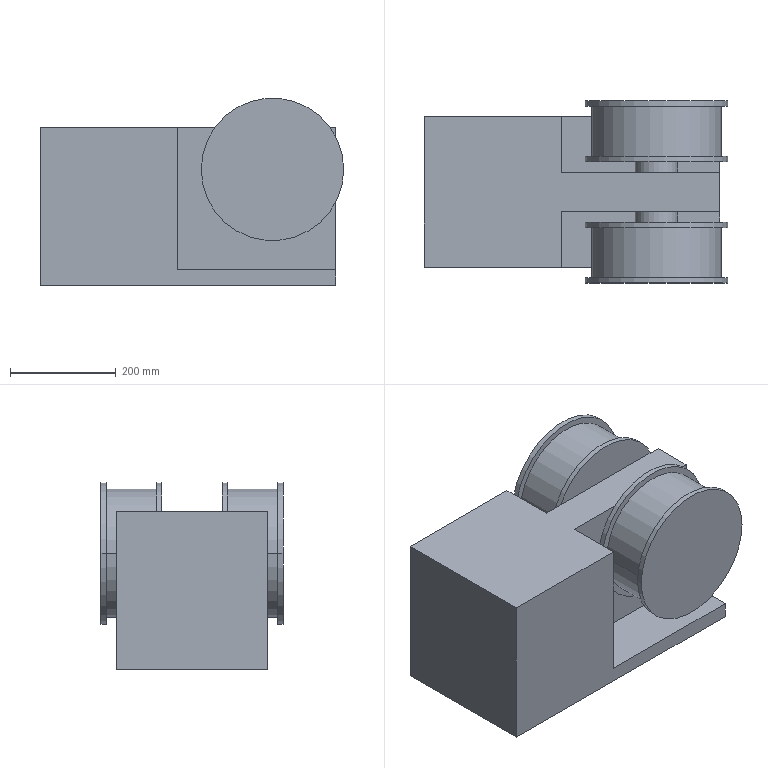Part | NX | features BREP 1 | 1 solid | 36 faces | box 575 x 345 x 355 mm | volume 42318553 mm3 | plane 20 | cylinder 16 | commonest cylinder face diameters 270 x8 80 x4 245 x4
STEP:
#1=CARTESIAN_POINT('',(295.,172.5,220.));
#2=VERTEX_POINT('',#1);
#3=CARTESIAN_POINT('',(25.,172.5,220.));
#4=VERTEX_POINT('',#3);
#5=CARTESIAN_POINT('',(160.,172.5,220.));
#6=DIRECTION('',(0.,-1.,0.));
#7=DIRECTION('',(1.,0.,0.));
#8=AXIS2_PLACEMENT_3D('',#5,#6,#7);
#9=CIRCLE('',#8,135.);
#10=EDGE_CURVE('',#2,#4,#9,.T.);
#11=ORIENTED_EDGE('',*,*,#10,.T.);
#12=CARTESIAN_POINT('',(25.,162.5,220.));
#13=VERTEX_POINT('',#12);
#14=CARTESIAN_POINT('',(25.,172.5,220.));
#15=DIRECTION('',(0.,-1.,0.));
#16=VECTOR('',#15,1000.);
#17=LINE('',#14,#16);
#18=EDGE_CURVE('',#13,#4,#17,.F.);
#19=ORIENTED_EDGE('',*,*,#18,.F.);
#20=CARTESIAN_POINT('',(295.,162.5,220.));
#21=VERTEX_POINT('',#20);
#22=CARTESIAN_POINT('',(160.,162.5,220.));
#23=DIRECTION('',(0.,-1.,0.));
#24=DIRECTION('',(1.,0.,0.));
#25=AXIS2_PLACEMENT_3D('',#22,#23,#24);
#26=CIRCLE('',#25,135.);
#27=EDGE_CURVE('',#21,#13,#26,.T.);
#28=ORIENTED_EDGE('',*,*,#27,.F.);
#29=CARTESIAN_POINT('',(295.,172.5,220.));
#30=DIRECTION('',(0.,-1.,0.));
#31=VECTOR('',#30,1000.);
#32=LINE('',#29,#31);
#33=EDGE_CURVE('',#21,#2,#32,.F.);
#34=ORIENTED_EDGE('',*,*,#33,.T.);
#35=EDGE_LOOP('',(#11,#19,#28,#34));
#36=FACE_BOUND('',#35,.T.);
#37=CARTESIAN_POINT('',(160.,172.5,220.));
#38=DIRECTION('',(0.,-1.,0.));
#39=DIRECTION('',(1.,0.,0.));
#40=AXIS2_PLACEMENT_3D('',#37,#38,#39);
#41=CYLINDRICAL_SURFACE('',#40,135.);
#42=ADVANCED_FACE('',(#36),#41,.T.);
#43=CARTESIAN_POINT('',(282.5,162.5,220.));
#44=VERTEX_POINT('',#43);
#45=CARTESIAN_POINT('',(37.5,162.5,220.));
#46=VERTEX_POINT('',#45);
#47=CARTESIAN_POINT('',(160.,162.5,220.));
#48=DIRECTION('',(0.,-1.,0.));
#49=DIRECTION('',(1.,0.,0.));
#50=AXIS2_PLACEMENT_3D('',#47,#48,#49);
#51=CIRCLE('',#50,122.5);
#52=EDGE_CURVE('',#44,#46,#51,.T.);
#53=ORIENTED_EDGE('',*,*,#52,.T.);
#54=CARTESIAN_POINT('',(37.5,67.5,220.));
#55=VERTEX_POINT('',#54);
#56=CARTESIAN_POINT('',(37.5,162.5,220.));
#57=DIRECTION('',(0.,-1.,0.));
#58=VECTOR('',#57,1000.);
#59=LINE('',#56,#58);
#60=EDGE_CURVE('',#55,#46,#59,.F.);
#61=ORIENTED_EDGE('',*,*,#60,.F.);
#62=CARTESIAN_POINT('',(282.5,67.5,220.));
#63=VERTEX_POINT('',#62);
#64=CARTESIAN_POINT('',(160.,67.5,220.));
#65=DIRECTION('',(0.,-1.,0.));
#66=DIRECTION('',(1.,0.,0.));
#67=AXIS2_PLACEMENT_3D('',#64,#65,#66);
#68=CIRCLE('',#67,122.5);
#69=EDGE_CURVE('',#63,#55,#68,.T.);
#70=ORIENTED_EDGE('',*,*,#69,.F.);
#71=CARTESIAN_POINT('',(282.5,162.5,220.));
#72=DIRECTION('',(0.,-1.,0.));
#73=VECTOR('',#72,1000.);
#74=LINE('',#71,#73);
#75=EDGE_CURVE('',#63,#44,#74,.F.);
#76=ORIENTED_EDGE('',*,*,#75,.T.);
#77=EDGE_LOOP('',(#53,#61,#70,#76));
#78=FACE_BOUND('',#77,.T.);
#79=CARTESIAN_POINT('',(160.,162.5,220.));
#80=DIRECTION('',(0.,-1.,0.));
#81=DIRECTION('',(1.,0.,0.));
#82=AXIS2_PLACEMENT_3D('',#79,#80,#81);
#83=CYLINDRICAL_SURFACE('',#82,122.5);
#84=ADVANCED_FACE('',(#78),#83,.T.);
#85=CARTESIAN_POINT('',(295.,67.5,220.));
#86=VERTEX_POINT('',#85);
#87=CARTESIAN_POINT('',(25.,67.5,220.));
#88=VERTEX_POINT('',#87);
#89=CARTESIAN_POINT('',(160.,67.5,220.));
#90=DIRECTION('',(0.,-1.,0.));
#91=DIRECTION('',(1.,0.,0.));
#92=AXIS2_PLACEMENT_3D('',#89,#90,#91);
#93=CIRCLE('',#92,135.);
#94=EDGE_CURVE('',#86,#88,#93,.T.);
#95=ORIENTED_EDGE('',*,*,#94,.T.);
#96=CARTESIAN_POINT('',(25.,57.5,220.));
#97=VERTEX_POINT('',#96);
#98=CARTESIAN_POINT('',(25.,67.5,220.));
#99=DIRECTION('',(0.,-1.,0.));
#100=VECTOR('',#99,1000.);
#101=LINE('',#98,#100);
#102=EDGE_CURVE('',#97,#88,#101,.F.);
#103=ORIENTED_EDGE('',*,*,#102,.F.);
#104=CARTESIAN_POINT('',(295.,57.5,220.));
#105=VERTEX_POINT('',#104);
#106=CARTESIAN_POINT('',(160.,57.5,220.));
#107=DIRECTION('',(0.,-1.,0.));
#108=DIRECTION('',(1.,0.,0.));
#109=AXIS2_PLACEMENT_3D('',#106,#107,#108);
#110=CIRCLE('',#109,135.);
#111=EDGE_CURVE('',#105,#97,#110,.T.);
#112=ORIENTED_EDGE('',*,*,#111,.F.);
#113=CARTESIAN_POINT('',(295.,67.5,220.));
#114=DIRECTION('',(0.,-1.,0.));
#115=VECTOR('',#114,1000.);
#116=LINE('',#113,#115);
#117=EDGE_CURVE('',#105,#86,#116,.F.);
#118=ORIENTED_EDGE('',*,*,#117,.T.);
#119=EDGE_LOOP('',(#95,#103,#112,#118));
#120=FACE_BOUND('',#119,.T.);
#121=CARTESIAN_POINT('',(160.,67.5,220.));
#122=DIRECTION('',(0.,-1.,0.));
#123=DIRECTION('',(1.,0.,0.));
#124=AXIS2_PLACEMENT_3D('',#121,#122,#123);
#125=CYLINDRICAL_SURFACE('',#124,135.);
#126=ADVANCED_FACE('',(#120),#125,.T.);
#127=CARTESIAN_POINT('',(200.,57.5,220.));
#128=VERTEX_POINT('',#127);
#129=CARTESIAN_POINT('',(120.,57.5,220.));
#130=VERTEX_POINT('',#129);
#131=CARTESIAN_POINT('',(160.,57.5,220.));
#132=DIRECTION('',(0.,-1.,0.));
#133=DIRECTION('',(1.,0.,0.));
#134=AXIS2_PLACEMENT_3D('',#131,#132,#133);
#135=CIRCLE('',#134,40.);
#136=EDGE_CURVE('',#128,#130,#135,.T.);
#137=ORIENTED_EDGE('',*,*,#136,.T.);
#138=CARTESIAN_POINT('',(120.,37.5,220.));
#139=VERTEX_POINT('',#138);
#140=CARTESIAN_POINT('',(120.,57.5,220.));
#141=DIRECTION('',(0.,-1.,0.));
#142=VECTOR('',#141,1000.);
#143=LINE('',#140,#142);
#144=EDGE_CURVE('',#139,#130,#143,.F.);
#145=ORIENTED_EDGE('',*,*,#144,.F.);
#146=CARTESIAN_POINT('',(200.,37.5,220.));
#147=VERTEX_POINT('',#146);
#148=CARTESIAN_POINT('',(160.,37.5,220.));
#149=DIRECTION('',(0.,-1.,0.));
#150=DIRECTION('',(1.,0.,0.));
#151=AXIS2_PLACEMENT_3D('',#148,#149,#150);
#152=CIRCLE('',#151,40.);
#153=EDGE_CURVE('',#147,#139,#152,.T.);
#154=ORIENTED_EDGE('',*,*,#153,.F.);
#155=CARTESIAN_POINT('',(200.,57.5,220.));
#156=DIRECTION('',(0.,-1.,0.));
#157=VECTOR('',#156,1000.);
#158=LINE('',#155,#157);
#159=EDGE_CURVE('',#147,#128,#158,.F.);
#160=ORIENTED_EDGE('',*,*,#159,.T.);
#161=EDGE_LOOP('',(#137,#145,#154,#160));
#162=FACE_BOUND('',#161,.T.);
#163=CARTESIAN_POINT('',(160.,57.5,220.));
#164=DIRECTION('',(0.,-1.,0.));
#165=DIRECTION('',(1.,0.,0.));
#166=AXIS2_PLACEMENT_3D('',#163,#164,#165);
#167=CYLINDRICAL_SURFACE('',#166,40.);
#168=ADVANCED_FACE('',(#162),#167,.T.);
#169=CARTESIAN_POINT('',(295.,-172.5,220.));
#170=VERTEX_POINT('',#169);
#171=CARTESIAN_POINT('',(25.,-172.5,220.));
#172=VERTEX_POINT('',#171);
#173=CARTESIAN_POINT('',(160.,-172.5,220.));
#174=DIRECTION('',(0.,-1.,0.));
#175=DIRECTION('',(1.,0.,0.));
#176=AXIS2_PLACEMENT_3D('',#173,#174,#175);
#177=CIRCLE('',#176,135.);
#178=EDGE_CURVE('',#170,#172,#177,.T.);
#179=ORIENTED_EDGE('',*,*,#178,.F.);
#180=CARTESIAN_POINT('',(295.,-162.5,220.));
#181=VERTEX_POINT('',#180);
#182=CARTESIAN_POINT('',(295.,-172.5,220.));
#183=DIRECTION('',(0.,1.,0.));
#184=VECTOR('',#183,1000.);
#185=LINE('',#182,#184);
#186=EDGE_CURVE('',#170,#181,#185,.T.);
#187=ORIENTED_EDGE('',*,*,#186,.T.);
#188=CARTESIAN_POINT('',(25.,-162.5,220.));
#189=VERTEX_POINT('',#188);
#190=CARTESIAN_POINT('',(160.,-162.5,220.));
#191=DIRECTION('',(0.,-1.,0.));
#192=DIRECTION('',(1.,0.,0.));
#193=AXIS2_PLACEMENT_3D('',#190,#191,#192);
#194=CIRCLE('',#193,135.);
#195=EDGE_CURVE('',#181,#189,#194,.T.);
#196=ORIENTED_EDGE('',*,*,#195,.T.);
#197=CARTESIAN_POINT('',(25.,-172.5,220.));
#198=DIRECTION('',(0.,1.,0.));
#199=VECTOR('',#198,1000.);
#200=LINE('',#197,#199);
#201=EDGE_CURVE('',#172,#189,#200,.T.);
#202=ORIENTED_EDGE('',*,*,#201,.F.);
#203=EDGE_LOOP('',(#179,#187,#196,#202));
#204=FACE_BOUND('',#203,.T.);
#205=CARTESIAN_POINT('',(160.,-172.5,220.));
#206=DIRECTION('',(0.,1.,0.));
#207=DIRECTION('',(-1.,0.,0.));
#208=AXIS2_PLACEMENT_3D('',#205,#206,#207);
#209=CYLINDRICAL_SURFACE('',#208,135.);
#210=ADVANCED_FACE('',(#204),#209,.T.);
#211=CARTESIAN_POINT('',(282.5,-162.5,220.));
#212=VERTEX_POINT('',#211);
#213=CARTESIAN_POINT('',(37.5,-162.5,220.));
#214=VERTEX_POINT('',#213);
#215=CARTESIAN_POINT('',(160.,-162.5,220.));
#216=DIRECTION('',(0.,-1.,0.));
#217=DIRECTION('',(1.,0.,0.));
#218=AXIS2_PLACEMENT_3D('',#215,#216,#217);
#219=CIRCLE('',#218,122.5);
#220=EDGE_CURVE('',#212,#214,#219,.T.);
#221=ORIENTED_EDGE('',*,*,#220,.F.);
#222=CARTESIAN_POINT('',(282.5,-67.5,220.));
#223=VERTEX_POINT('',#222);
#224=CARTESIAN_POINT('',(282.5,-162.5,220.));
#225=DIRECTION('',(0.,1.,0.));
#226=VECTOR('',#225,1000.);
#227=LINE('',#224,#226);
#228=EDGE_CURVE('',#212,#223,#227,.T.);
#229=ORIENTED_EDGE('',*,*,#228,.T.);
#230=CARTESIAN_POINT('',(37.5,-67.5,220.));
#231=VERTEX_POINT('',#230);
#232=CARTESIAN_POINT('',(160.,-67.5,220.));
#233=DIRECTION('',(0.,-1.,0.));
#234=DIRECTION('',(1.,0.,0.));
#235=AXIS2_PLACEMENT_3D('',#232,#233,#234);
#236=CIRCLE('',#235,122.5);
#237=EDGE_CURVE('',#223,#231,#236,.T.);
#238=ORIENTED_EDGE('',*,*,#237,.T.);
#239=CARTESIAN_POINT('',(37.5,-162.5,220.));
#240=DIRECTION('',(0.,1.,0.));
#241=VECTOR('',#240,1000.);
#242=LINE('',#239,#241);
#243=EDGE_CURVE('',#214,#231,#242,.T.);
#244=ORIENTED_EDGE('',*,*,#243,.F.);
#245=EDGE_LOOP('',(#221,#229,#238,#244));
#246=FACE_BOUND('',#245,.T.);
#247=CARTESIAN_POINT('',(160.,-162.5,220.));
#248=DIRECTION('',(0.,1.,0.));
#249=DIRECTION('',(-1.,0.,0.));
#250=AXIS2_PLACEMENT_3D('',#247,#248,#249);
#251=CYLINDRICAL_SURFACE('',#250,122.5);
#252=ADVANCED_FACE('',(#246),#251,.T.);
#253=CARTESIAN_POINT('',(295.,-67.5,220.));
#254=VERTEX_POINT('',#253);
#255=CARTESIAN_POINT('',(25.,-67.5,220.));
#256=VERTEX_POINT('',#255);
#257=CARTESIAN_POINT('',(160.,-67.5,220.));
#258=DIRECTION('',(0.,-1.,0.));
#259=DIRECTION('',(1.,0.,0.));
#260=AXIS2_PLACEMENT_3D('',#257,#258,#259);
#261=CIRCLE('',#260,135.);
#262=EDGE_CURVE('',#254,#256,#261,.T.);
#263=ORIENTED_EDGE('',*,*,#262,.F.);
#264=CARTESIAN_POINT('',(295.,-57.5,220.));
#265=VERTEX_POINT('',#264);
#266=CARTESIAN_POINT('',(295.,-67.5,220.));
#267=DIRECTION('',(0.,1.,0.));
#268=VECTOR('',#267,1000.);
#269=LINE('',#266,#268);
#270=EDGE_CURVE('',#254,#265,#269,.T.);
#271=ORIENTED_EDGE('',*,*,#270,.T.);
#272=CARTESIAN_POINT('',(25.,-57.5,220.));
#273=VERTEX_POINT('',#272);
#274=CARTESIAN_POINT('',(160.,-57.5,220.));
#275=DIRECTION('',(0.,-1.,0.));
#276=DIRECTION('',(1.,0.,0.));
#277=AXIS2_PLACEMENT_3D('',#274,#275,#276);
#278=CIRCLE('',#277,135.);
#279=EDGE_CURVE('',#265,#273,#278,.T.);
#280=ORIENTED_EDGE('',*,*,#279,.T.);
#281=CARTESIAN_POINT('',(25.,-67.5,220.));
#282=DIRECTION('',(0.,1.,0.));
#283=VECTOR('',#282,1000.);
#284=LINE('',#281,#283);
#285=EDGE_CURVE('',#256,#273,#284,.T.);
#286=ORIENTED_EDGE('',*,*,#285,.F.);
#287=EDGE_LOOP('',(#263,#271,#280,#286));
#288=FACE_BOUND('',#287,.T.);
#289=CARTESIAN_POINT('',(160.,-67.5,220.));
#290=DIRECTION('',(0.,1.,0.));
#291=DIRECTION('',(-1.,0.,0.));
#292=AXIS2_PLACEMENT_3D('',#289,#290,#291);
#293=CYLINDRICAL_SURFACE('',#292,135.);
#294=ADVANCED_FACE('',(#288),#293,.T.);
#295=CARTESIAN_POINT('',(200.,-57.5,220.));
#296=VERTEX_POINT('',#295);
#297=CARTESIAN_POINT('',(120.,-57.5,220.));
#298=VERTEX_POINT('',#297);
#299=CARTESIAN_POINT('',(160.,-57.5,220.));
#300=DIRECTION('',(0.,-1.,0.));
#301=DIRECTION('',(1.,0.,0.));
#302=AXIS2_PLACEMENT_3D('',#299,#300,#301);
#303=CIRCLE('',#302,40.);
#304=EDGE_CURVE('',#296,#298,#303,.T.);
#305=ORIENTED_EDGE('',*,*,#304,.F.);
#306=CARTESIAN_POINT('',(200.,-37.5,220.));
#307=VERTEX_POINT('',#306);
#308=CARTESIAN_POINT('',(200.,-57.5,220.));
#309=DIRECTION('',(0.,1.,0.));
#310=VECTOR('',#309,1000.);
#311=LINE('',#308,#310);
#312=EDGE_CURVE('',#296,#307,#311,.T.);
#313=ORIENTED_EDGE('',*,*,#312,.T.);
#314=CARTESIAN_POINT('',(120.,-37.5,220.));
#315=VERTEX_POINT('',#314);
#316=CARTESIAN_POINT('',(160.,-37.5,220.));
#317=DIRECTION('',(0.,-1.,0.));
#318=DIRECTION('',(-1.,0.,0.));
#319=AXIS2_PLACEMENT_3D('',#316,#317,#318);
#320=CIRCLE('',#319,40.);
#321=EDGE_CURVE('',#307,#315,#320,.T.);
#322=ORIENTED_EDGE('',*,*,#321,.T.);
#323=CARTESIAN_POINT('',(120.,-57.5,220.));
#324=DIRECTION('',(0.,1.,0.));
#325=VECTOR('',#324,1000.);
#326=LINE('',#323,#325);
#327=EDGE_CURVE('',#298,#315,#326,.T.);
#328=ORIENTED_EDGE('',*,*,#327,.F.);
#329=EDGE_LOOP('',(#305,#313,#322,#328));
#330=FACE_BOUND('',#329,.T.);
#331=CARTESIAN_POINT('',(160.,-57.5,220.));
#332=DIRECTION('',(0.,1.,0.));
#333=DIRECTION('',(-1.,0.,0.));
#334=AXIS2_PLACEMENT_3D('',#331,#332,#333);
#335=CYLINDRICAL_SURFACE('',#334,40.);
#336=ADVANCED_FACE('',(#330),#335,.T.);
#337=CARTESIAN_POINT('',(280.,37.5,30.));
#338=VERTEX_POINT('',#337);
#339=CARTESIAN_POINT('',(280.,142.5,30.));
#340=VERTEX_POINT('',#339);
#341=CARTESIAN_POINT('',(280.,142.5,30.));
#342=DIRECTION('',(0.,1.,0.));
#343=VECTOR('',#342,1000.);
#344=LINE('',#341,#343);
#345=EDGE_CURVE('',#338,#340,#344,.T.);
#346=ORIENTED_EDGE('',*,*,#345,.F.);
#347=CARTESIAN_POINT('',(280.,37.5,300.));
#348=VERTEX_POINT('',#347);
#349=CARTESIAN_POINT('',(280.,37.5,30.));
#350=DIRECTION('',(0.,0.,1.));
#351=VECTOR('',#350,1000.);
#352=LINE('',#349,#351);
#353=EDGE_CURVE('',#338,#348,#352,.T.);
#354=ORIENTED_EDGE('',*,*,#353,.T.);
#355=CARTESIAN_POINT('',(280.,-37.5,300.));
#356=VERTEX_POINT('',#355);
#357=CARTESIAN_POINT('',(280.,-142.5,300.));
#358=DIRECTION('',(0.,1.,0.));
#359=VECTOR('',#358,1000.);
#360=LINE('',#357,#359);
#361=EDGE_CURVE('',#356,#348,#360,.T.);
#362=ORIENTED_EDGE('',*,*,#361,.F.);
#363=CARTESIAN_POINT('',(280.,-37.5,30.));
#364=VERTEX_POINT('',#363);
#365=CARTESIAN_POINT('',(280.,-37.5,30.));
#366=DIRECTION('',(0.,0.,1.));
#367=VECTOR('',#366,1000.);
#368=LINE('',#365,#367);
#369=EDGE_CURVE('',#364,#356,#368,.T.);
#370=ORIENTED_EDGE('',*,*,#369,.F.);
#371=CARTESIAN_POINT('',(280.,-142.5,30.));
#372=VERTEX_POINT('',#371);
#373=CARTESIAN_POINT('',(280.,-142.5,30.));
#374=DIRECTION('',(0.,1.,0.));
#375=VECTOR('',#374,1000.);
#376=LINE('',#373,#375);
#377=EDGE_CURVE('',#372,#364,#376,.T.);
#378=ORIENTED_EDGE('',*,*,#377,.F.);
#379=CARTESIAN_POINT('',(280.,-142.5,0.));
#380=VERTEX_POINT('',#379);
#381=CARTESIAN_POINT('',(280.,-142.5,300.));
#382=DIRECTION('',(0.,0.,-1.));
#383=VECTOR('',#382,1000.);
#384=LINE('',#381,#383);
#385=EDGE_CURVE('',#372,#380,#384,.T.);
#386=ORIENTED_EDGE('',*,*,#385,.T.);
#387=CARTESIAN_POINT('',(280.,142.5,0.));
#388=VERTEX_POINT('',#387);
#389=CARTESIAN_POINT('',(280.,-142.5,0.));
#390=DIRECTION('',(0.,1.,0.));
#391=VECTOR('',#390,1000.);
#392=LINE('',#389,#391);
#393=EDGE_CURVE('',#380,#388,#392,.T.);
#394=ORIENTED_EDGE('',*,*,#393,.T.);
#395=CARTESIAN_POINT('',(280.,142.5,300.));
#396=DIRECTION('',(0.,0.,-1.));
#397=VECTOR('',#396,1000.);
#398=LINE('',#395,#397);
#399=EDGE_CURVE('',#340,#388,#398,.T.);
#400=ORIENTED_EDGE('',*,*,#399,.F.);
#401=EDGE_LOOP('',(#346,#354,#362,#370,#378,#386,#394,#400));
#402=FACE_BOUND('',#401,.T.);
#403=CARTESIAN_POINT('',(280.,-142.5,300.));
#404=DIRECTION('',(-1.,0.,0.));
#405=DIRECTION('',(0.,0.,1.));
#406=AXIS2_PLACEMENT_3D('',#403,#404,#405);
#407=PLANE('',#406);
#408=ADVANCED_FACE('',(#402),#407,.F.);
#409=CARTESIAN_POINT('',(-20.,142.5,300.));
#410=VERTEX_POINT('',#409);
#411=CARTESIAN_POINT('',(-280.,142.5,300.));
#412=VERTEX_POINT('',#411);
#413=CARTESIAN_POINT('',(-280.,142.5,300.));
#414=DIRECTION('',(-1.,0.,0.));
#415=VECTOR('',#414,1000.);
#416=LINE('',#413,#415);
#417=EDGE_CURVE('',#410,#412,#416,.T.);
#418=ORIENTED_EDGE('',*,*,#417,.F.);
#419=CARTESIAN_POINT('',(-20.,142.5,30.));
#420=VERTEX_POINT('',#419);
#421=CARTESIAN_POINT('',(-20.,142.5,30.));
#422=DIRECTION('',(0.,0.,1.));
#423=VECTOR('',#422,1000.);
#424=LINE('',#421,#423);
#425=EDGE_CURVE('',#420,#410,#424,.T.);
#426=ORIENTED_EDGE('',*,*,#425,.F.);
#427=CARTESIAN_POINT('',(280.,142.5,30.));
#428=DIRECTION('',(-1.,0.,0.));
#429=VECTOR('',#428,1000.);
#430=LINE('',#427,#429);
#431=EDGE_CURVE('',#340,#420,#430,.T.);
#432=ORIENTED_EDGE('',*,*,#431,.F.);
#433=ORIENTED_EDGE('',*,*,#399,.T.);
#434=CARTESIAN_POINT('',(-280.,142.5,0.));
#435=VERTEX_POINT('',#434);
#436=CARTESIAN_POINT('',(-280.,142.5,0.));
#437=DIRECTION('',(-1.,0.,0.));
#438=VECTOR('',#437,1000.);
#439=LINE('',#436,#438);
#440=EDGE_CURVE('',#388,#435,#439,.T.);
#441=ORIENTED_EDGE('',*,*,#440,.T.);
#442=CARTESIAN_POINT('',(-280.,142.5,300.));
#443=DIRECTION('',(0.,0.,-1.));
#444=VECTOR('',#443,1000.);
#445=LINE('',#442,#444);
#446=EDGE_CURVE('',#412,#435,#445,.T.);
#447=ORIENTED_EDGE('',*,*,#446,.F.);
#448=EDGE_LOOP('',(#418,#426,#432,#433,#441,#447));
#449=FACE_BOUND('',#448,.T.);
#450=CARTESIAN_POINT('',(-280.,142.5,300.));
#451=DIRECTION('',(0.,-1.,0.));
#452=DIRECTION('',(0.,0.,-1.));
#453=AXIS2_PLACEMENT_3D('',#450,#451,#452);
#454=PLANE('',#453);
#455=ADVANCED_FACE('',(#449),#454,.F.);
#456=CARTESIAN_POINT('',(-280.,-142.5,0.));
#457=VERTEX_POINT('',#456);
#458=CARTESIAN_POINT('',(-280.,-142.5,0.));
#459=DIRECTION('',(0.,-1.,0.));
#460=VECTOR('',#459,1000.);
#461=LINE('',#458,#460);
#462=EDGE_CURVE('',#435,#457,#461,.T.);
#463=ORIENTED_EDGE('',*,*,#462,.T.);
#464=CARTESIAN_POINT('',(-280.,-142.5,300.));
#465=VERTEX_POINT('',#464);
#466=CARTESIAN_POINT('',(-280.,-142.5,300.));
#467=DIRECTION('',(0.,0.,-1.));
#468=VECTOR('',#467,1000.);
#469=LINE('',#466,#468);
#470=EDGE_CURVE('',#465,#457,#469,.T.);
#471=ORIENTED_EDGE('',*,*,#470,.F.);
#472=CARTESIAN_POINT('',(-280.,-142.5,300.));
#473=DIRECTION('',(0.,-1.,0.));
#474=VECTOR('',#473,1000.);
#475=LINE('',#472,#474);
#476=EDGE_CURVE('',#412,#465,#475,.T.);
#477=ORIENTED_EDGE('',*,*,#476,.F.);
#478=ORIENTED_EDGE('',*,*,#446,.T.);
#479=EDGE_LOOP('',(#463,#471,#477,#478));
#480=FACE_BOUND('',#479,.T.);
#481=CARTESIAN_POINT('',(-280.,-142.5,300.));
#482=DIRECTION('',(1.,0.,0.));
#483=DIRECTION('',(0.,1.,0.));
#484=AXIS2_PLACEMENT_3D('',#481,#482,#483);
#485=PLANE('',#484);
#486=ADVANCED_FACE('',(#480),#485,.F.);
#487=CARTESIAN_POINT('',(-20.,-142.5,30.));
#488=VERTEX_POINT('',#487);
#489=CARTESIAN_POINT('',(280.,-142.5,30.));
#490=DIRECTION('',(1.,0.,0.));
#491=VECTOR('',#490,1000.);
#492=LINE('',#489,#491);
#493=EDGE_CURVE('',#488,#372,#492,.T.);
#494=ORIENTED_EDGE('',*,*,#493,.F.);
#495=CARTESIAN_POINT('',(-20.,-142.5,300.));
#496=VERTEX_POINT('',#495);
#497=CARTESIAN_POINT('',(-20.,-142.5,30.));
#498=DIRECTION('',(0.,0.,1.));
#499=VECTOR('',#498,1000.);
#500=LINE('',#497,#499);
#501=EDGE_CURVE('',#488,#496,#500,.T.);
#502=ORIENTED_EDGE('',*,*,#501,.T.);
#503=CARTESIAN_POINT('',(-280.,-142.5,300.));
#504=DIRECTION('',(1.,0.,0.));
#505=VECTOR('',#504,1000.);
#506=LINE('',#503,#505);
#507=EDGE_CURVE('',#465,#496,#506,.T.);
#508=ORIENTED_EDGE('',*,*,#507,.F.);
#509=ORIENTED_EDGE('',*,*,#470,.T.);
#510=CARTESIAN_POINT('',(-280.,-142.5,0.));
#511=DIRECTION('',(1.,0.,0.));
#512=VECTOR('',#511,1000.);
#513=LINE('',#510,#512);
#514=EDGE_CURVE('',#457,#380,#513,.T.);
#515=ORIENTED_EDGE('',*,*,#514,.T.);
#516=ORIENTED_EDGE('',*,*,#385,.F.);
#517=EDGE_LOOP('',(#494,#502,#508,#509,#515,#516));
#518=FACE_BOUND('',#517,.T.);
#519=CARTESIAN_POINT('',(-280.,-142.5,300.));
#520=DIRECTION('',(0.,1.,0.));
#521=DIRECTION('',(1.,0.,0.));
#522=AXIS2_PLACEMENT_3D('',#519,#520,#521);
#523=PLANE('',#522);
#524=ADVANCED_FACE('',(#518),#523,.F.);
#525=ORIENTED_EDGE('',*,*,#361,.T.);
#526=CARTESIAN_POINT('',(-20.,37.5,300.));
#527=VERTEX_POINT('',#526);
#528=CARTESIAN_POINT('',(280.,37.5,300.));
#529=DIRECTION('',(1.,0.,0.));
#530=VECTOR('',#529,1000.);
#531=LINE('',#528,#530);
#532=EDGE_CURVE('',#527,#348,#531,.T.);
#533=ORIENTED_EDGE('',*,*,#532,.F.);
#534=CARTESIAN_POINT('',(-20.,142.5,300.));
#535=DIRECTION('',(0.,-1.,0.));
#536=VECTOR('',#535,1000.);
#537=LINE('',#534,#536);
#538=EDGE_CURVE('',#410,#527,#537,.T.);
#539=ORIENTED_EDGE('',*,*,#538,.F.);
#540=ORIENTED_EDGE('',*,*,#417,.T.);
#541=ORIENTED_EDGE('',*,*,#476,.T.);
#542=ORIENTED_EDGE('',*,*,#507,.T.);
#543=CARTESIAN_POINT('',(-20.,-37.5,300.));
#544=VERTEX_POINT('',#543);
#545=CARTESIAN_POINT('',(-20.,-142.5,300.));
#546=DIRECTION('',(0.,-1.,0.));
#547=VECTOR('',#546,1000.);
#548=LINE('',#545,#547);
#549=EDGE_CURVE('',#544,#496,#548,.T.);
#550=ORIENTED_EDGE('',*,*,#549,.F.);
#551=CARTESIAN_POINT('',(280.,-37.5,300.));
#552=DIRECTION('',(-1.,0.,0.));
#553=VECTOR('',#552,1000.);
#554=LINE('',#551,#553);
#555=EDGE_CURVE('',#356,#544,#554,.T.);
#556=ORIENTED_EDGE('',*,*,#555,.F.);
#557=EDGE_LOOP('',(#525,#533,#539,#540,#541,#542,#550,#556));
#558=FACE_BOUND('',#557,.T.);
#559=CARTESIAN_POINT('',(0.,0.,300.));
#560=DIRECTION('',(0.,0.,-1.));
#561=DIRECTION('',(0.,-1.,0.));
#562=AXIS2_PLACEMENT_3D('',#559,#560,#561);
#563=PLANE('',#562);
#564=ADVANCED_FACE('',(#558),#563,.F.);
#565=ORIENTED_EDGE('',*,*,#393,.F.);
#566=ORIENTED_EDGE('',*,*,#514,.F.);
#567=ORIENTED_EDGE('',*,*,#462,.F.);
#568=ORIENTED_EDGE('',*,*,#440,.F.);
#569=EDGE_LOOP('',(#565,#566,#567,#568));
#570=FACE_BOUND('',#569,.T.);
#571=CARTESIAN_POINT('',(0.,0.,0.));
#572=DIRECTION('',(0.,0.,-1.));
#573=DIRECTION('',(0.,-1.,0.));
#574=AXIS2_PLACEMENT_3D('',#571,#572,#573);
#575=PLANE('',#574);
#576=ADVANCED_FACE('',(#570),#575,.T.);
#577=ORIENTED_EDGE('',*,*,#549,.T.);
#578=ORIENTED_EDGE('',*,*,#501,.F.);
#579=CARTESIAN_POINT('',(-20.,-37.5,30.));
#580=VERTEX_POINT('',#579);
#581=CARTESIAN_POINT('',(-20.,-142.5,30.));
#582=DIRECTION('',(0.,-1.,0.));
#583=VECTOR('',#582,1000.);
#584=LINE('',#581,#583);
#585=EDGE_CURVE('',#580,#488,#584,.T.);
#586=ORIENTED_EDGE('',*,*,#585,.F.);
#587=CARTESIAN_POINT('',(-20.,-37.5,30.));
#588=DIRECTION('',(0.,0.,1.));
#589=VECTOR('',#588,1000.);
#590=LINE('',#587,#589);
#591=EDGE_CURVE('',#580,#544,#590,.T.);
#592=ORIENTED_EDGE('',*,*,#591,.T.);
#593=EDGE_LOOP('',(#577,#578,#586,#592));
#594=FACE_BOUND('',#593,.T.);
#595=CARTESIAN_POINT('',(-20.,-142.5,30.));
#596=DIRECTION('',(-1.,0.,0.));
#597=DIRECTION('',(0.,0.,1.));
#598=AXIS2_PLACEMENT_3D('',#595,#596,#597);
#599=PLANE('',#598);
#600=ADVANCED_FACE('',(#594),#599,.F.);
#601=ORIENTED_EDGE('',*,*,#555,.T.);
#602=ORIENTED_EDGE('',*,*,#591,.F.);
#603=CARTESIAN_POINT('',(280.,-37.5,30.));
#604=DIRECTION('',(-1.,0.,0.));
#605=VECTOR('',#604,1000.);
#606=LINE('',#603,#605);
#607=EDGE_CURVE('',#364,#580,#606,.T.);
#608=ORIENTED_EDGE('',*,*,#607,.F.);
#609=ORIENTED_EDGE('',*,*,#369,.T.);
#610=EDGE_LOOP('',(#601,#602,#608,#609));
#611=FACE_BOUND('',#610,.T.);
#612=CARTESIAN_POINT('',(160.,-37.5,220.));
#613=DIRECTION('',(0.,-1.,0.));
#614=DIRECTION('',(-1.,0.,0.));
#615=AXIS2_PLACEMENT_3D('',#612,#613,#614);
#616=CIRCLE('',#615,40.);
#617=EDGE_CURVE('',#315,#307,#616,.T.);
#618=ORIENTED_EDGE('',*,*,#617,.F.);
#619=ORIENTED_EDGE('',*,*,#321,.F.);
#620=EDGE_LOOP('',(#618,#619));
#621=FACE_BOUND('',#620,.T.);
#622=CARTESIAN_POINT('',(280.,-37.5,30.));
#623=DIRECTION('',(0.,1.,0.));
#624=DIRECTION('',(1.,0.,0.));
#625=AXIS2_PLACEMENT_3D('',#622,#623,#624);
#626=PLANE('',#625);
#627=ADVANCED_FACE('',(#611,#621),#626,.F.);
#628=ORIENTED_EDGE('',*,*,#377,.T.);
#629=ORIENTED_EDGE('',*,*,#607,.T.);
#630=ORIENTED_EDGE('',*,*,#585,.T.);
#631=ORIENTED_EDGE('',*,*,#493,.T.);
#632=EDGE_LOOP('',(#628,#629,#630,#631));
#633=FACE_BOUND('',#632,.T.);
#634=CARTESIAN_POINT('',(0.,0.,30.));
#635=DIRECTION('',(0.,0.,1.));
#636=DIRECTION('',(1.,0.,0.));
#637=AXIS2_PLACEMENT_3D('',#634,#635,#636);
#638=PLANE('',#637);
#639=ADVANCED_FACE('',(#633),#638,.T.);
#640=ORIENTED_EDGE('',*,*,#532,.T.);
#641=ORIENTED_EDGE('',*,*,#353,.F.);
#642=CARTESIAN_POINT('',(-20.,37.5,30.));
#643=VERTEX_POINT('',#642);
#644=CARTESIAN_POINT('',(280.,37.5,30.));
#645=DIRECTION('',(1.,0.,0.));
#646=VECTOR('',#645,1000.);
#647=LINE('',#644,#646);
#648=EDGE_CURVE('',#643,#338,#647,.T.);
#649=ORIENTED_EDGE('',*,*,#648,.F.);
#650=CARTESIAN_POINT('',(-20.,37.5,30.));
#651=DIRECTION('',(0.,0.,1.));
#652=VECTOR('',#651,1000.);
#653=LINE('',#650,#652);
#654=EDGE_CURVE('',#643,#527,#653,.T.);
#655=ORIENTED_EDGE('',*,*,#654,.T.);
#656=EDGE_LOOP('',(#640,#641,#649,#655));
#657=FACE_BOUND('',#656,.T.);
#658=ORIENTED_EDGE('',*,*,#153,.T.);
#659=CARTESIAN_POINT('',(160.,37.5,220.));
#660=DIRECTION('',(0.,-1.,0.));
#661=DIRECTION('',(1.,0.,0.));
#662=AXIS2_PLACEMENT_3D('',#659,#660,#661);
#663=CIRCLE('',#662,40.);
#664=EDGE_CURVE('',#139,#147,#663,.T.);
#665=ORIENTED_EDGE('',*,*,#664,.T.);
#666=EDGE_LOOP('',(#658,#665));
#667=FACE_BOUND('',#666,.T.);
#668=CARTESIAN_POINT('',(280.,37.5,30.));
#669=DIRECTION('',(0.,-1.,0.));
#670=DIRECTION('',(0.,0.,-1.));
#671=AXIS2_PLACEMENT_3D('',#668,#669,#670);
#672=PLANE('',#671);
#673=ADVANCED_FACE('',(#657,#667),#672,.F.);
#674=ORIENTED_EDGE('',*,*,#538,.T.);
#675=ORIENTED_EDGE('',*,*,#654,.F.);
#676=CARTESIAN_POINT('',(-20.,142.5,30.));
#677=DIRECTION('',(0.,-1.,0.));
#678=VECTOR('',#677,1000.);
#679=LINE('',#676,#678);
#680=EDGE_CURVE('',#420,#643,#679,.T.);
#681=ORIENTED_EDGE('',*,*,#680,.F.);
#682=ORIENTED_EDGE('',*,*,#425,.T.);
#683=EDGE_LOOP('',(#674,#675,#681,#682));
#684=FACE_BOUND('',#683,.T.);
#685=CARTESIAN_POINT('',(-20.,142.5,30.));
#686=DIRECTION('',(-1.,0.,0.));
#687=DIRECTION('',(0.,1.,0.));
#688=AXIS2_PLACEMENT_3D('',#685,#686,#687);
#689=PLANE('',#688);
#690=ADVANCED_FACE('',(#684),#689,.F.);
#691=ORIENTED_EDGE('',*,*,#345,.T.);
#692=ORIENTED_EDGE('',*,*,#431,.T.);
#693=ORIENTED_EDGE('',*,*,#680,.T.);
#694=ORIENTED_EDGE('',*,*,#648,.T.);
#695=EDGE_LOOP('',(#691,#692,#693,#694));
#696=FACE_BOUND('',#695,.T.);
#697=CARTESIAN_POINT('',(0.,0.,30.));
#698=DIRECTION('',(0.,0.,-1.));
#699=DIRECTION('',(0.,-1.,0.));
#700=AXIS2_PLACEMENT_3D('',#697,#698,#699);
#701=PLANE('',#700);
#702=ADVANCED_FACE('',(#696),#701,.F.);
#703=ORIENTED_EDGE('',*,*,#312,.F.);
#704=CARTESIAN_POINT('',(160.,-57.5,220.));
#705=DIRECTION('',(0.,-1.,0.));
#706=DIRECTION('',(1.,0.,0.));
#707=AXIS2_PLACEMENT_3D('',#704,#705,#706);
#708=CIRCLE('',#707,40.);
#709=EDGE_CURVE('',#298,#296,#708,.T.);
#710=ORIENTED_EDGE('',*,*,#709,.F.);
#711=ORIENTED_EDGE('',*,*,#327,.T.);
#712=ORIENTED_EDGE('',*,*,#617,.T.);
#713=EDGE_LOOP('',(#703,#710,#711,#712));
#714=FACE_BOUND('',#713,.T.);
#715=CARTESIAN_POINT('',(160.,-57.5,220.));
#716=DIRECTION('',(0.,1.,0.));
#717=DIRECTION('',(-1.,0.,0.));
#718=AXIS2_PLACEMENT_3D('',#715,#716,#717);
#719=CYLINDRICAL_SURFACE('',#718,40.);
#720=ADVANCED_FACE('',(#714),#719,.T.);
#721=ORIENTED_EDGE('',*,*,#270,.F.);
#722=CARTESIAN_POINT('',(160.,-67.5,220.));
#723=DIRECTION('',(0.,-1.,0.));
#724=DIRECTION('',(1.,0.,0.));
#725=AXIS2_PLACEMENT_3D('',#722,#723,#724);
#726=CIRCLE('',#725,135.);
#727=EDGE_CURVE('',#256,#254,#726,.T.);
#728=ORIENTED_EDGE('',*,*,#727,.F.);
#729=ORIENTED_EDGE('',*,*,#285,.T.);
#730=CARTESIAN_POINT('',(160.,-57.5,220.));
#731=DIRECTION('',(0.,-1.,0.));
#732=DIRECTION('',(1.,0.,0.));
#733=AXIS2_PLACEMENT_3D('',#730,#731,#732);
#734=CIRCLE('',#733,135.);
#735=EDGE_CURVE('',#273,#265,#734,.T.);
#736=ORIENTED_EDGE('',*,*,#735,.T.);
#737=EDGE_LOOP('',(#721,#728,#729,#736));
#738=FACE_BOUND('',#737,.T.);
#739=CARTESIAN_POINT('',(160.,-67.5,220.));
#740=DIRECTION('',(0.,1.,0.));
#741=DIRECTION('',(-1.,0.,0.));
#742=AXIS2_PLACEMENT_3D('',#739,#740,#741);
#743=CYLINDRICAL_SURFACE('',#742,135.);
#744=ADVANCED_FACE('',(#738),#743,.T.);
#745=ORIENTED_EDGE('',*,*,#727,.T.);
#746=ORIENTED_EDGE('',*,*,#262,.T.);
#747=EDGE_LOOP('',(#745,#746));
#748=FACE_BOUND('',#747,.T.);
#749=CARTESIAN_POINT('',(160.,-67.5,220.));
#750=DIRECTION('',(0.,-1.,0.));
#751=DIRECTION('',(1.,0.,0.));
#752=AXIS2_PLACEMENT_3D('',#749,#750,#751);
#753=CIRCLE('',#752,122.5);
#754=EDGE_CURVE('',#231,#223,#753,.T.);
#755=ORIENTED_EDGE('',*,*,#754,.F.);
#756=ORIENTED_EDGE('',*,*,#237,.F.);
#757=EDGE_LOOP('',(#755,#756));
#758=FACE_BOUND('',#757,.T.);
#759=CARTESIAN_POINT('',(160.,-67.5,220.));
#760=DIRECTION('',(0.,-1.,0.));
#761=DIRECTION('',(-1.,0.,0.));
#762=AXIS2_PLACEMENT_3D('',#759,#760,#761);
#763=PLANE('',#762);
#764=ADVANCED_FACE('',(#748,#758),#763,.T.);
#765=ORIENTED_EDGE('',*,*,#735,.F.);
#766=ORIENTED_EDGE('',*,*,#279,.F.);
#767=EDGE_LOOP('',(#765,#766));
#768=FACE_BOUND('',#767,.T.);
#769=ORIENTED_EDGE('',*,*,#709,.T.);
#770=ORIENTED_EDGE('',*,*,#304,.T.);
#771=EDGE_LOOP('',(#769,#770));
#772=FACE_BOUND('',#771,.T.);
#773=CARTESIAN_POINT('',(160.,-57.5,220.));
#774=DIRECTION('',(0.,-1.,0.));
#775=DIRECTION('',(-1.,0.,0.));
#776=AXIS2_PLACEMENT_3D('',#773,#774,#775);
#777=PLANE('',#776);
#778=ADVANCED_FACE('',(#768,#772),#777,.F.);
#779=ORIENTED_EDGE('',*,*,#228,.F.);
#780=CARTESIAN_POINT('',(160.,-162.5,220.));
#781=DIRECTION('',(0.,-1.,0.));
#782=DIRECTION('',(1.,0.,0.));
#783=AXIS2_PLACEMENT_3D('',#780,#781,#782);
#784=CIRCLE('',#783,122.5);
#785=EDGE_CURVE('',#214,#212,#784,.T.);
#786=ORIENTED_EDGE('',*,*,#785,.F.);
#787=ORIENTED_EDGE('',*,*,#243,.T.);
#788=ORIENTED_EDGE('',*,*,#754,.T.);
#789=EDGE_LOOP('',(#779,#786,#787,#788));
#790=FACE_BOUND('',#789,.T.);
#791=CARTESIAN_POINT('',(160.,-162.5,220.));
#792=DIRECTION('',(0.,1.,0.));
#793=DIRECTION('',(-1.,0.,0.));
#794=AXIS2_PLACEMENT_3D('',#791,#792,#793);
#795=CYLINDRICAL_SURFACE('',#794,122.5);
#796=ADVANCED_FACE('',(#790),#795,.T.);
#797=ORIENTED_EDGE('',*,*,#186,.F.);
#798=CARTESIAN_POINT('',(160.,-172.5,220.));
#799=DIRECTION('',(0.,-1.,0.));
#800=DIRECTION('',(1.,0.,0.));
#801=AXIS2_PLACEMENT_3D('',#798,#799,#800);
#802=CIRCLE('',#801,135.);
#803=EDGE_CURVE('',#172,#170,#802,.T.);
#804=ORIENTED_EDGE('',*,*,#803,.F.);
#805=ORIENTED_EDGE('',*,*,#201,.T.);
#806=CARTESIAN_POINT('',(160.,-162.5,220.));
#807=DIRECTION('',(0.,-1.,0.));
#808=DIRECTION('',(1.,0.,0.));
#809=AXIS2_PLACEMENT_3D('',#806,#807,#808);
#810=CIRCLE('',#809,135.);
#811=EDGE_CURVE('',#189,#181,#810,.T.);
#812=ORIENTED_EDGE('',*,*,#811,.T.);
#813=EDGE_LOOP('',(#797,#804,#805,#812));
#814=FACE_BOUND('',#813,.T.);
#815=CARTESIAN_POINT('',(160.,-172.5,220.));
#816=DIRECTION('',(0.,1.,0.));
#817=DIRECTION('',(-1.,0.,0.));
#818=AXIS2_PLACEMENT_3D('',#815,#816,#817);
#819=CYLINDRICAL_SURFACE('',#818,135.);
#820=ADVANCED_FACE('',(#814),#819,.T.);
#821=ORIENTED_EDGE('',*,*,#803,.T.);
#822=ORIENTED_EDGE('',*,*,#178,.T.);
#823=EDGE_LOOP('',(#821,#822));
#824=FACE_BOUND('',#823,.T.);
#825=CARTESIAN_POINT('',(160.,-172.5,220.));
#826=DIRECTION('',(0.,-1.,0.));
#827=DIRECTION('',(-1.,0.,0.));
#828=AXIS2_PLACEMENT_3D('',#825,#826,#827);
#829=PLANE('',#828);
#830=ADVANCED_FACE('',(#824),#829,.T.);
#831=ORIENTED_EDGE('',*,*,#811,.F.);
#832=ORIENTED_EDGE('',*,*,#195,.F.);
#833=EDGE_LOOP('',(#831,#832));
#834=FACE_BOUND('',#833,.T.);
#835=ORIENTED_EDGE('',*,*,#785,.T.);
#836=ORIENTED_EDGE('',*,*,#220,.T.);
#837=EDGE_LOOP('',(#835,#836));
#838=FACE_BOUND('',#837,.T.);
#839=CARTESIAN_POINT('',(160.,-162.5,220.));
#840=DIRECTION('',(0.,-1.,0.));
#841=DIRECTION('',(-1.,0.,0.));
#842=AXIS2_PLACEMENT_3D('',#839,#840,#841);
#843=PLANE('',#842);
#844=ADVANCED_FACE('',(#834,#838),#843,.F.);
#845=ORIENTED_EDGE('',*,*,#144,.T.);
#846=CARTESIAN_POINT('',(160.,57.5,220.));
#847=DIRECTION('',(0.,-1.,0.));
#848=DIRECTION('',(1.,0.,0.));
#849=AXIS2_PLACEMENT_3D('',#846,#847,#848);
#850=CIRCLE('',#849,40.);
#851=EDGE_CURVE('',#130,#128,#850,.T.);
#852=ORIENTED_EDGE('',*,*,#851,.T.);
#853=ORIENTED_EDGE('',*,*,#159,.F.);
#854=ORIENTED_EDGE('',*,*,#664,.F.);
#855=EDGE_LOOP('',(#845,#852,#853,#854));
#856=FACE_BOUND('',#855,.T.);
#857=CARTESIAN_POINT('',(160.,57.5,220.));
#858=DIRECTION('',(0.,-1.,0.));
#859=DIRECTION('',(1.,0.,0.));
#860=AXIS2_PLACEMENT_3D('',#857,#858,#859);
#861=CYLINDRICAL_SURFACE('',#860,40.);
#862=ADVANCED_FACE('',(#856),#861,.T.);
#863=ORIENTED_EDGE('',*,*,#102,.T.);
#864=CARTESIAN_POINT('',(160.,67.5,220.));
#865=DIRECTION('',(0.,-1.,0.));
#866=DIRECTION('',(1.,0.,0.));
#867=AXIS2_PLACEMENT_3D('',#864,#865,#866);
#868=CIRCLE('',#867,135.);
#869=EDGE_CURVE('',#88,#86,#868,.T.);
#870=ORIENTED_EDGE('',*,*,#869,.T.);
#871=ORIENTED_EDGE('',*,*,#117,.F.);
#872=CARTESIAN_POINT('',(160.,57.5,220.));
#873=DIRECTION('',(0.,-1.,0.));
#874=DIRECTION('',(1.,0.,0.));
#875=AXIS2_PLACEMENT_3D('',#872,#873,#874);
#876=CIRCLE('',#875,135.);
#877=EDGE_CURVE('',#97,#105,#876,.T.);
#878=ORIENTED_EDGE('',*,*,#877,.F.);
#879=EDGE_LOOP('',(#863,#870,#871,#878));
#880=FACE_BOUND('',#879,.T.);
#881=CARTESIAN_POINT('',(160.,67.5,220.));
#882=DIRECTION('',(0.,-1.,0.));
#883=DIRECTION('',(1.,0.,0.));
#884=AXIS2_PLACEMENT_3D('',#881,#882,#883);
#885=CYLINDRICAL_SURFACE('',#884,135.);
#886=ADVANCED_FACE('',(#880),#885,.T.);
#887=ORIENTED_EDGE('',*,*,#94,.F.);
#888=ORIENTED_EDGE('',*,*,#869,.F.);
#889=EDGE_LOOP('',(#887,#888));
#890=FACE_BOUND('',#889,.T.);
#891=ORIENTED_EDGE('',*,*,#69,.T.);
#892=CARTESIAN_POINT('',(160.,67.5,220.));
#893=DIRECTION('',(0.,-1.,0.));
#894=DIRECTION('',(1.,0.,0.));
#895=AXIS2_PLACEMENT_3D('',#892,#893,#894);
#896=CIRCLE('',#895,122.5);
#897=EDGE_CURVE('',#55,#63,#896,.T.);
#898=ORIENTED_EDGE('',*,*,#897,.T.);
#899=EDGE_LOOP('',(#891,#898));
#900=FACE_BOUND('',#899,.T.);
#901=CARTESIAN_POINT('',(160.,67.5,220.));
#902=DIRECTION('',(0.,1.,0.));
#903=DIRECTION('',(1.,0.,0.));
#904=AXIS2_PLACEMENT_3D('',#901,#902,#903);
#905=PLANE('',#904);
#906=ADVANCED_FACE('',(#890,#900),#905,.T.);
#907=ORIENTED_EDGE('',*,*,#111,.T.);
#908=ORIENTED_EDGE('',*,*,#877,.T.);
#909=EDGE_LOOP('',(#907,#908));
#910=FACE_BOUND('',#909,.T.);
#911=ORIENTED_EDGE('',*,*,#136,.F.);
#912=ORIENTED_EDGE('',*,*,#851,.F.);
#913=EDGE_LOOP('',(#911,#912));
#914=FACE_BOUND('',#913,.T.);
#915=CARTESIAN_POINT('',(160.,57.5,220.));
#916=DIRECTION('',(0.,1.,0.));
#917=DIRECTION('',(1.,0.,0.));
#918=AXIS2_PLACEMENT_3D('',#915,#916,#917);
#919=PLANE('',#918);
#920=ADVANCED_FACE('',(#910,#914),#919,.F.);
#921=ORIENTED_EDGE('',*,*,#60,.T.);
#922=CARTESIAN_POINT('',(160.,162.5,220.));
#923=DIRECTION('',(0.,-1.,0.));
#924=DIRECTION('',(1.,0.,0.));
#925=AXIS2_PLACEMENT_3D('',#922,#923,#924);
#926=CIRCLE('',#925,122.5);
#927=EDGE_CURVE('',#46,#44,#926,.T.);
#928=ORIENTED_EDGE('',*,*,#927,.T.);
#929=ORIENTED_EDGE('',*,*,#75,.F.);
#930=ORIENTED_EDGE('',*,*,#897,.F.);
#931=EDGE_LOOP('',(#921,#928,#929,#930));
#932=FACE_BOUND('',#931,.T.);
#933=CARTESIAN_POINT('',(160.,162.5,220.));
#934=DIRECTION('',(0.,-1.,0.));
#935=DIRECTION('',(1.,0.,0.));
#936=AXIS2_PLACEMENT_3D('',#933,#934,#935);
#937=CYLINDRICAL_SURFACE('',#936,122.5);
#938=ADVANCED_FACE('',(#932),#937,.T.);
#939=ORIENTED_EDGE('',*,*,#18,.T.);
#940=CARTESIAN_POINT('',(160.,172.5,220.));
#941=DIRECTION('',(0.,-1.,0.));
#942=DIRECTION('',(1.,0.,0.));
#943=AXIS2_PLACEMENT_3D('',#940,#941,#942);
#944=CIRCLE('',#943,135.);
#945=EDGE_CURVE('',#4,#2,#944,.T.);
#946=ORIENTED_EDGE('',*,*,#945,.T.);
#947=ORIENTED_EDGE('',*,*,#33,.F.);
#948=CARTESIAN_POINT('',(160.,162.5,220.));
#949=DIRECTION('',(0.,-1.,0.));
#950=DIRECTION('',(1.,0.,0.));
#951=AXIS2_PLACEMENT_3D('',#948,#949,#950);
#952=CIRCLE('',#951,135.);
#953=EDGE_CURVE('',#13,#21,#952,.T.);
#954=ORIENTED_EDGE('',*,*,#953,.F.);
#955=EDGE_LOOP('',(#939,#946,#947,#954));
#956=FACE_BOUND('',#955,.T.);
#957=CARTESIAN_POINT('',(160.,172.5,220.));
#958=DIRECTION('',(0.,-1.,0.));
#959=DIRECTION('',(1.,0.,0.));
#960=AXIS2_PLACEMENT_3D('',#957,#958,#959);
#961=CYLINDRICAL_SURFACE('',#960,135.);
#962=ADVANCED_FACE('',(#956),#961,.T.);
#963=ORIENTED_EDGE('',*,*,#10,.F.);
#964=ORIENTED_EDGE('',*,*,#945,.F.);
#965=EDGE_LOOP('',(#963,#964));
#966=FACE_BOUND('',#965,.T.);
#967=CARTESIAN_POINT('',(160.,172.5,220.));
#968=DIRECTION('',(0.,1.,0.));
#969=DIRECTION('',(1.,0.,0.));
#970=AXIS2_PLACEMENT_3D('',#967,#968,#969);
#971=PLANE('',#970);
#972=ADVANCED_FACE('',(#966),#971,.T.);
#973=ORIENTED_EDGE('',*,*,#27,.T.);
#974=ORIENTED_EDGE('',*,*,#953,.T.);
#975=EDGE_LOOP('',(#973,#974));
#976=FACE_BOUND('',#975,.T.);
#977=ORIENTED_EDGE('',*,*,#52,.F.);
#978=ORIENTED_EDGE('',*,*,#927,.F.);
#979=EDGE_LOOP('',(#977,#978));
#980=FACE_BOUND('',#979,.T.);
#981=CARTESIAN_POINT('',(160.,162.5,220.));
#982=DIRECTION('',(0.,1.,0.));
#983=DIRECTION('',(1.,0.,0.));
#984=AXIS2_PLACEMENT_3D('',#981,#982,#983);
#985=PLANE('',#984);
#986=ADVANCED_FACE('',(#976,#980),#985,.F.);
#987=CLOSED_SHELL('',(#42,#84,#126,#168,#210,#252,#294,#336,#408,#455,#486,#524,#564,#576,#600,#627,#639,#673,#690,#702,#720,#744,#764,#778,#796,#820,#830,#844,#862,#886,#906,#920,#938,#962,#972,#986));
#988=MANIFOLD_SOLID_BREP('',#987);
#989=(LENGTH_UNIT()NAMED_UNIT(*)SI_UNIT(.MILLI.,.METRE.));
#990=UNCERTAINTY_MEASURE_WITH_UNIT(LENGTH_MEASURE(0.00001),#989,'','');
#991=(NAMED_UNIT(*)PLANE_ANGLE_UNIT()SI_UNIT($,.RADIAN.));
#992=(NAMED_UNIT(*)SI_UNIT($,.STERADIAN.)SOLID_ANGLE_UNIT());
#993=(GEOMETRIC_REPRESENTATION_CONTEXT(3)GLOBAL_UNCERTAINTY_ASSIGNED_CONTEXT((#990))GLOBAL_UNIT_ASSIGNED_CONTEXT((#989,#991,#992))REPRESENTATION_CONTEXT('',''));
#994=ADVANCED_BREP_SHAPE_REPRESENTATION('',(#988),#993);